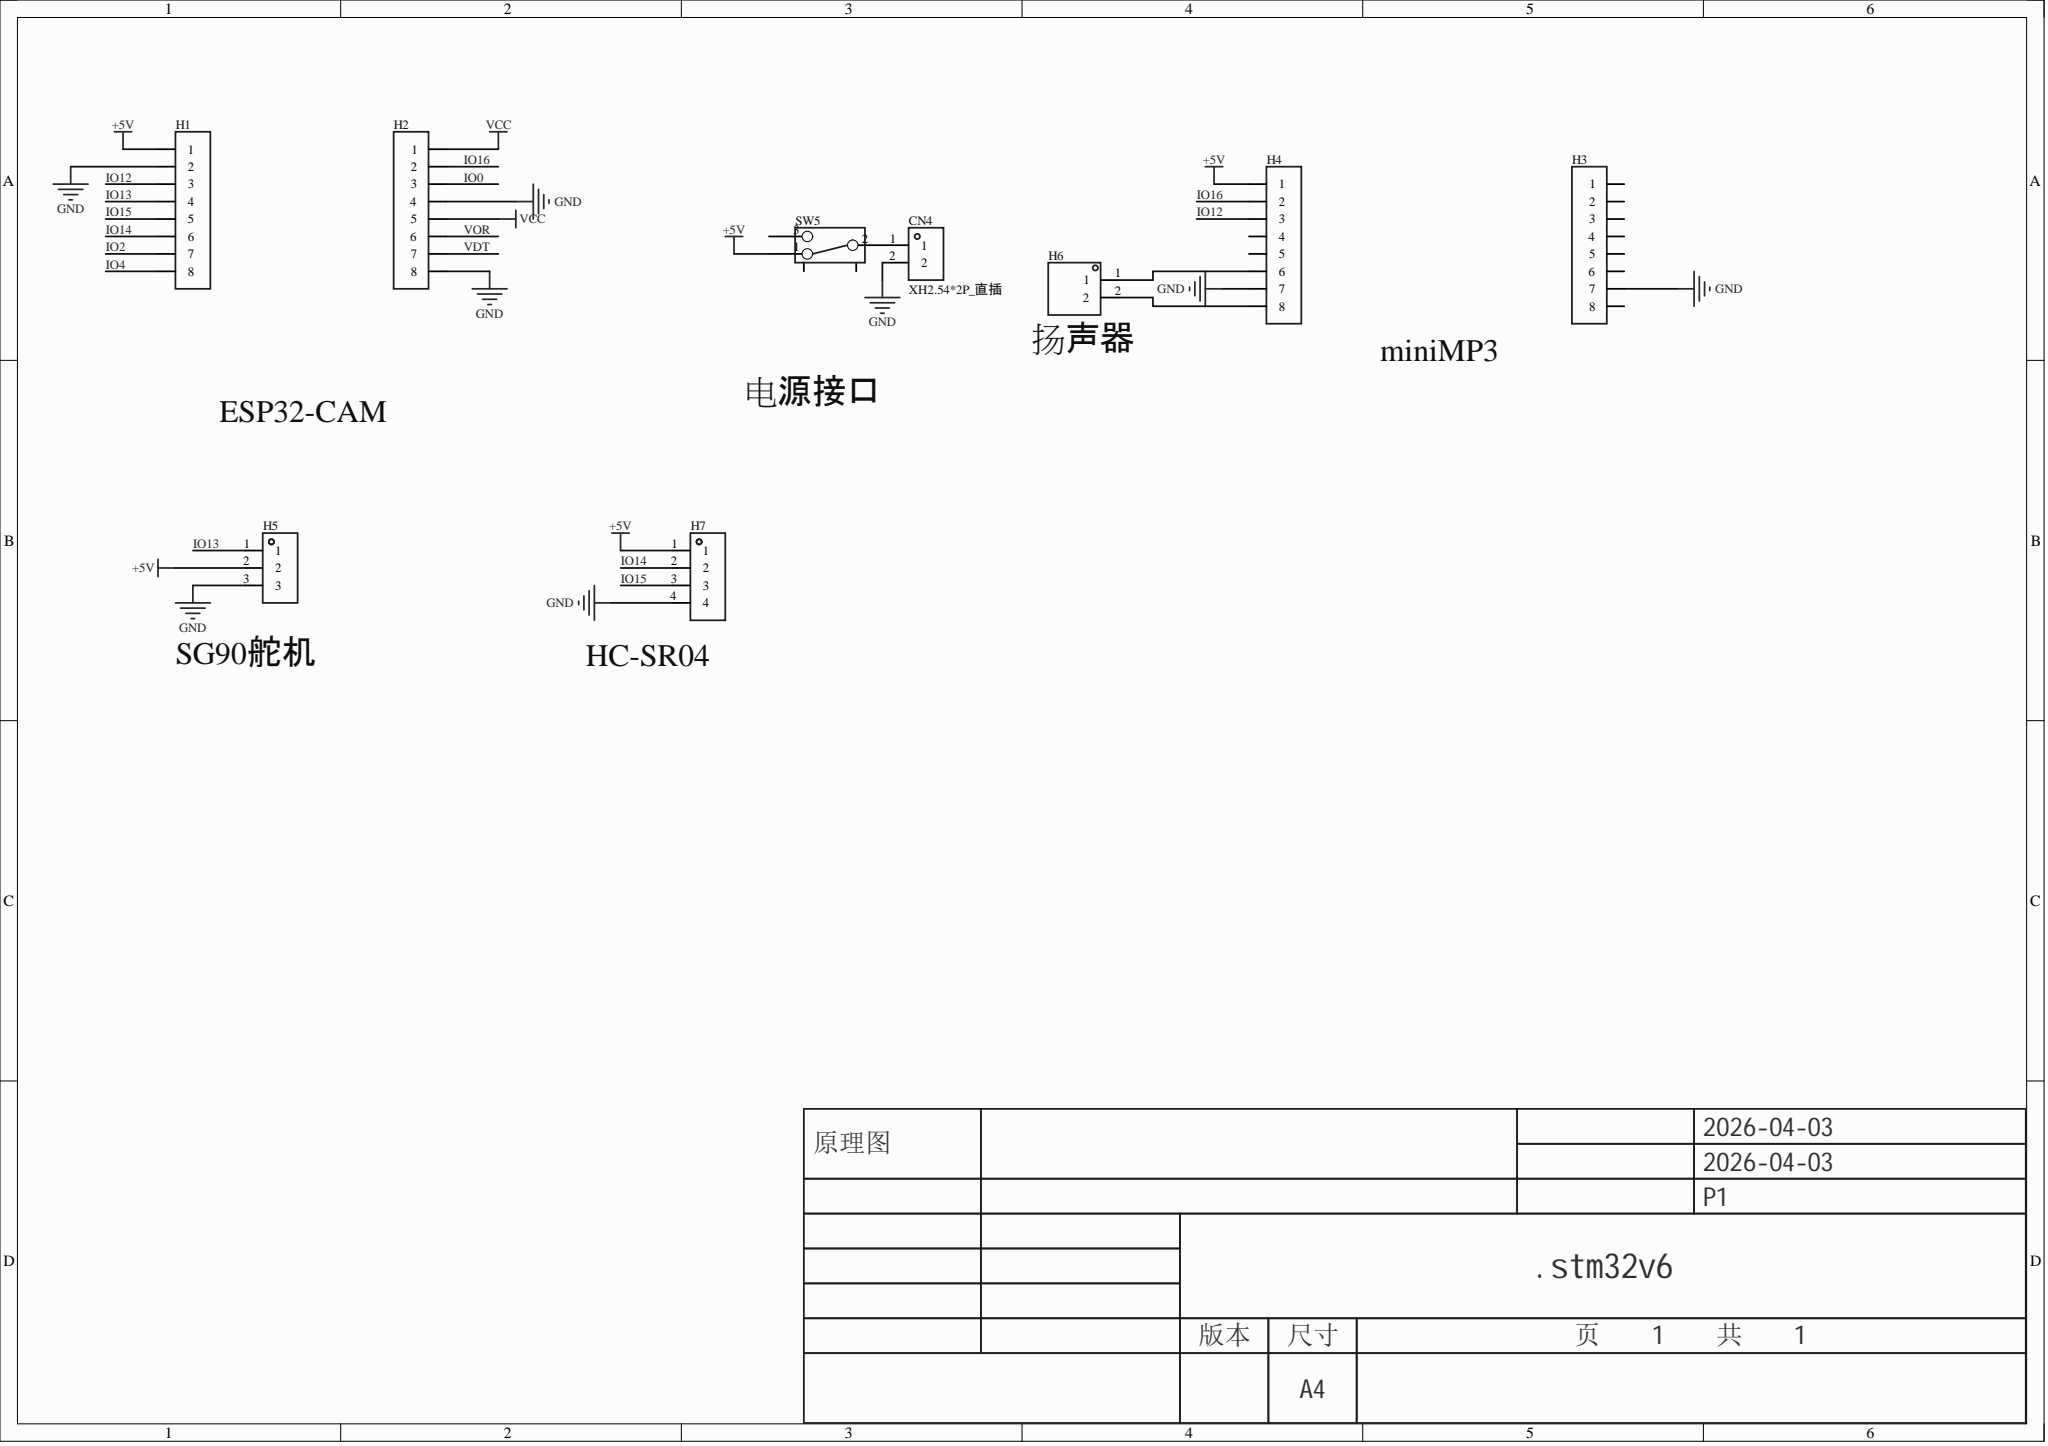Circuit board | Altium Designer | 9 parts | 11 nets
Bill of materials:
Comment,Description,Designator,Footprint,LibRef,Quantity
"XH2.54*2P_直插","","CN4","CONN-TH_2P-P2.50-XH2.54-2P","XH2.54*2P_直插","1"
"","","H1, H2, H3, H4","HDR-TH_8P-P2.54-V-F-1","HDR-F_2.54_1x8P","4"
"","","H5","HDR-TH_3P-P2.54-V-F","HDR-F_2.54_1x3P","1"
"","","H6","HDR-TH_2P-P2.54-V-M-1","HDR-M_2.54_1x2P","1"
"","","H7","HDR-TH_4P-P2.54-V-F","HDR-F_2.54_1x4P","1"
"","","SW5","拨动开关","拨动开关_正","1"
Netlist (Protel format):
[
CN4
CONN-TH_2P-P2.50-XH2.54-2P
XH2.54*2P_直插



]
[
H1
HDR-TH_8P-P2.54-V-F-1




]
[
H2
HDR-TH_8P-P2.54-V-F-1




]
[
H3
HDR-TH_8P-P2.54-V-F-1




]
[
H4
HDR-TH_8P-P2.54-V-F-1




]
[
H5
HDR-TH_3P-P2.54-V-F




]
[
H6
HDR-TH_2P-P2.54-V-M-1




]
[
H7
HDR-TH_4P-P2.54-V-F




]
[
SW5
拨动开关




]
(
VCC
H2-1
H2-5
)
(
NetH4_8
H4-8
H6-2
)
(
NetH4_6
H4-6
H6-1
)
(
NetCN4_1
CN4-1
SW5-2
)
(
IO16
H2-2
H4-2
)
(
IO15
H1-5
H7-3
)
(
IO14
H1-6
H7-2
)
(
IO13
H1-4
H5-1
)
(
IO12
H1-3
H4-3
)
(
GND
CN4-2
H1-2
H2-4
H2-8
H3-7
H4-7
H5-3
H7-4
)
(
+5V
H1-1
H4-1
H5-2
H7-1
SW5-1
)